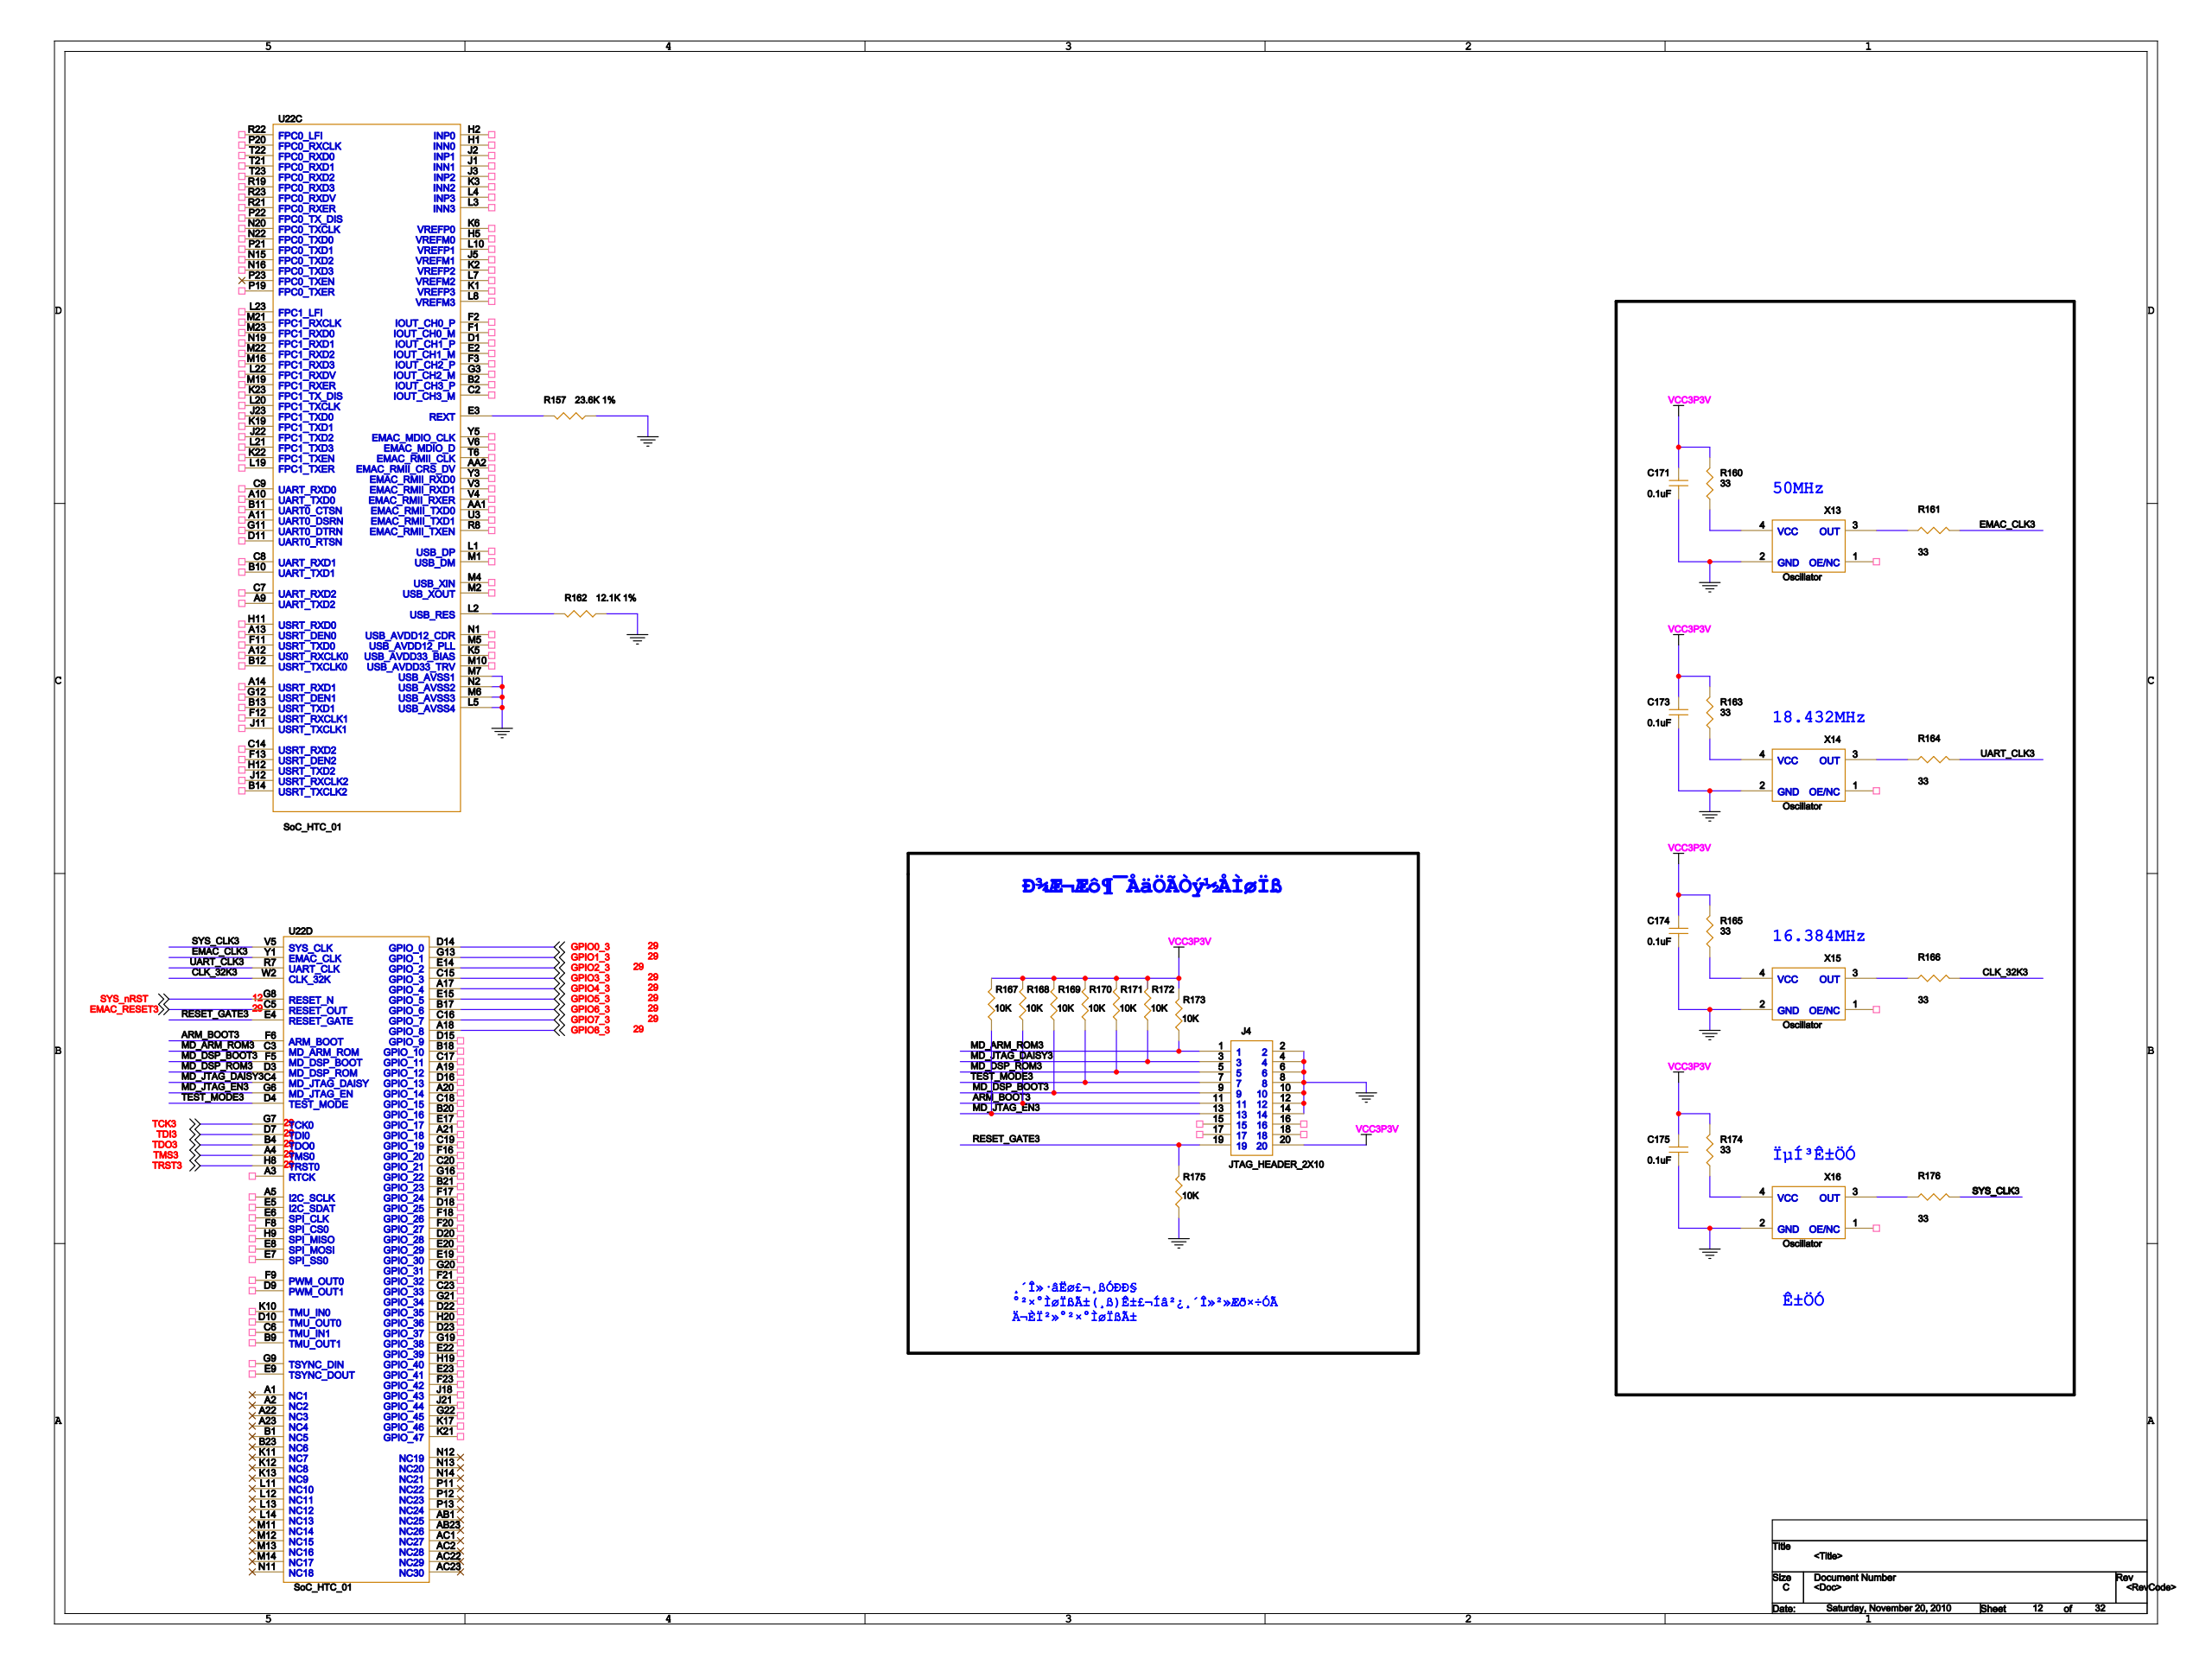Circuit board | Cadence Allegro | 1001 parts | 1318 nets | one sheet of the schematic
Parts on this sheet (reference | value | footprint):
C171 | 0.1uF | 0603
C173 | 0.1uF | 0603
C174 | 0.1uF | 0603
C175 | 0.1uF | 0603
J4 | JTAG_HEADER_2X10 | JTAG_HEADER_2X10
R157 | 23.6K 1% | 0603
R160 | 33 | 0603
R161 | 33 | 0603
R162 | 12.1K 1% | 0603
R163 | 33 | 0603
R164 | 33 | 0603
R165 | 33 | 0603
R166 | 33 | 0603
R167 | 10K | 0603
R168 | 10K | 0603
R169 | 10K | 0603
R170 | 10K | 0603
R171 | 10K | 0603
R172 | 10K | 0603
R173 | 10K | 0603
R174 | 33 | 0603
R175 | 10K | 0603
R176 | 33 | 0603
U22 | SoC_HTC_01 | L529_XIN
X13 | Oscillator | OSC_5_7
X14 | Oscillator | OSC_5_7
X15 | Oscillator | OSC_5_7
X16 | Oscillator | OSC_5_7
Nets of these parts (net: part-pin ...):
TDO3: U22-B4
TCK3: U22-G7
GPIO2_3: U22-E14
TDI3: U22-D7
TRST3: U22-H8
GPIO5_3: U22-E15
GPIO0_3: U22-D14
GPIO1_3: U22-G13
GPIO4_3: U22-A17
GPIO3_3: U22-C15
GPIO6_3: U22-B17
TMS3: U22-A4
EMAC_RESET3: U22-C5
GPIO7_3: U22-C16
GPIO8_3: U22-A18
GND: C171-2 C173-2 C174-2 C175-2 J4-2 J4-4 J4-6 J4-8 J4-10 J4-12 J4-14 R157-1 R162-1 R175-1 X13-2 X14-2 X15-2 X16-2 U22-L5 U22-M6 U22-M7 U22-N2
VCC3P3V: C171-1 C173-1 C174-1 C175-1 J4-20 R160-2 R163-2 R165-2 R167-2 R168-2 R169-2 R170-2 R171-2 R172-2 R173-2 R174-2 U22-J4
N16812845: R157-2 U22-E3
N16813063: R162-2 U22-L2
ARM_BOOT3: J4-11 R168-1 U22-F6
CLK_32K3: R166-2 U22-W2
EMAC_CLK3: R161-2 U22-Y1
MD_ARM_ROM3: J4-1 R173-1 U22-C3
MD_DSP_BOOT3: J4-9 R169-1 U22-F5
MD_DSP_ROM3: J4-5 R171-1 U22-D3
MD_JTAG_DAISY3: J4-3 R172-1 U22-C4
MD_JTAG_EN3: J4-13 R167-1 U22-G6
RESET_GATE3: J4-19 R175-2 U22-E4
SYS_CLK_16812641: R176-2 U22-V5
TEST_MODE3: J4-7 R170-1 U22-D4
UART_CLK3: R164-2 U22-R7
N16812405: R160-1 X13-4
N16812413: R161-1 X13-3
N16812423: R163-1 X14-4
N16812447: R164-1 X14-3
N16812596: R165-1 X15-4
N16812629: R166-1 X15-3
N16812637: R174-1 X16-4
N16812656: R176-1 X16-3